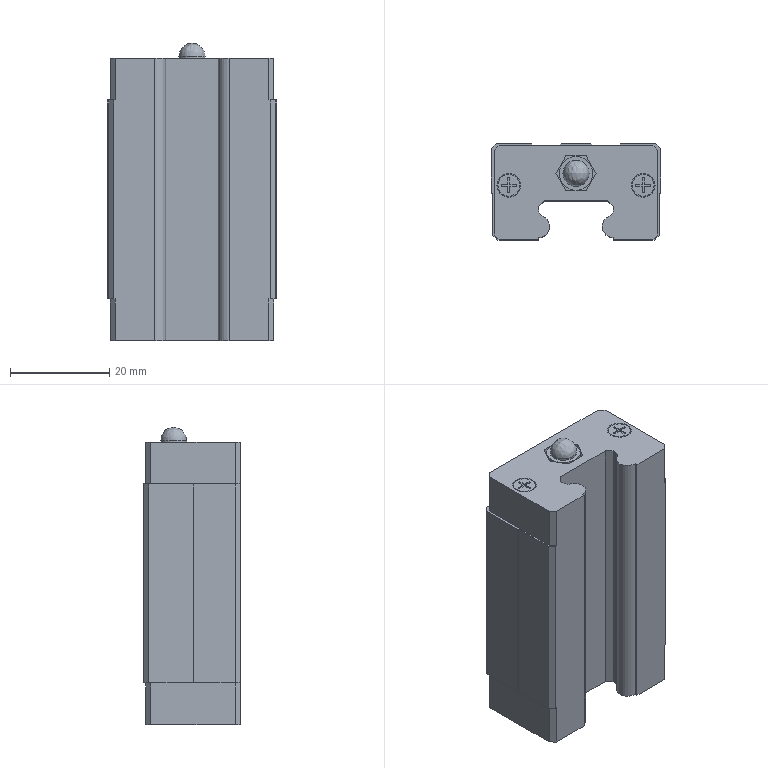Part | SolidWorks | features BaseBody 1 | 1 solid | 176 faces | box 34 x 19.4 x 59.8 mm | volume 30356 mm3 | plane 106 | cylinder 53 | cone 16 | spline 1 | commonest cylinder face diameters 3.08 x20 4.4 x11 3.242 x8 4.8 x8 3 x2 5.25 x2